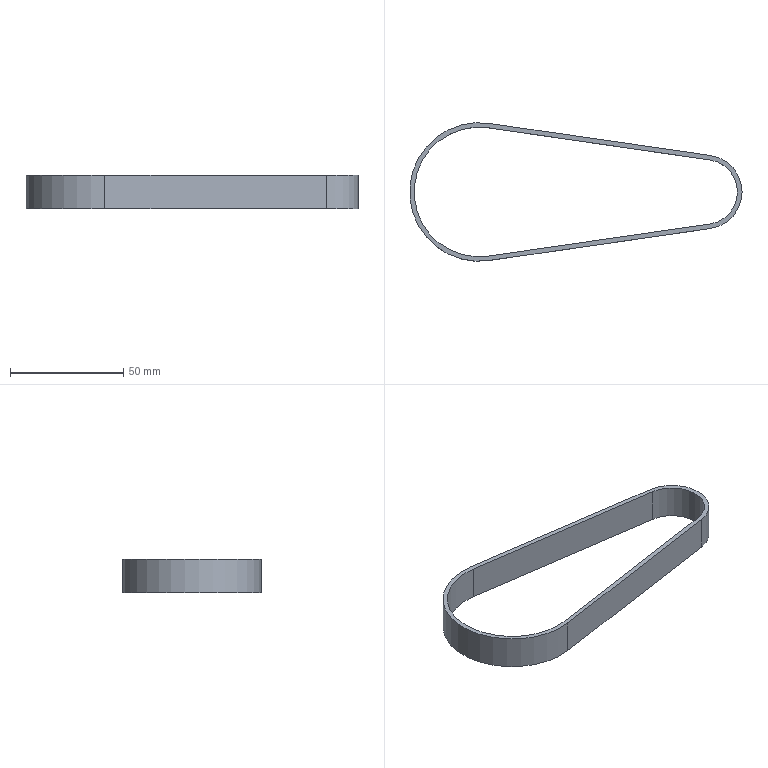Part | NX | 1 solid | 10 faces | box 146.965 x 61.3 x 15 mm | volume 10300 mm3 | plane 6 | cylinder 4 | commonest cylinder face diameters 28.63 x1 32.63 x1 57.3 x1 61.3 x1
STEP:
#1=CARTESIAN_POINT('',(102.339,-16.146,15.));
#2=VERTEX_POINT('',#1);
#3=CARTESIAN_POINT('',(102.339,16.146,15.));
#4=VERTEX_POINT('',#3);
#5=CARTESIAN_POINT('',(100.,0.,15.));
#6=DIRECTION('',(0.,0.,1.));
#7=DIRECTION('',(1.,0.,0.));
#8=AXIS2_PLACEMENT_3D('',#5,#6,#7);
#9=CIRCLE('',#8,16.315);
#10=EDGE_CURVE('',#2,#4,#9,.T.);
#11=ORIENTED_EDGE('',*,*,#10,.T.);
#12=CARTESIAN_POINT('',(4.394,30.333,15.));
#13=VERTEX_POINT('',#12);
#14=CARTESIAN_POINT('',(4.394,30.333,15.));
#15=DIRECTION('',(-0.9897,0.1434,0.));
#16=VECTOR('',#15,1000.);
#17=LINE('',#14,#16);
#18=EDGE_CURVE('',#4,#13,#17,.T.);
#19=ORIENTED_EDGE('',*,*,#18,.T.);
#20=CARTESIAN_POINT('',(4.394,-30.333,15.));
#21=VERTEX_POINT('',#20);
#22=CARTESIAN_POINT('',(0.,0.,15.));
#23=DIRECTION('',(0.,0.,1.));
#24=DIRECTION('',(1.,0.,0.));
#25=AXIS2_PLACEMENT_3D('',#22,#23,#24);
#26=CIRCLE('',#25,30.65);
#27=EDGE_CURVE('',#13,#21,#26,.T.);
#28=ORIENTED_EDGE('',*,*,#27,.T.);
#29=CARTESIAN_POINT('',(4.394,-30.333,15.));
#30=DIRECTION('',(0.9897,0.1434,0.));
#31=VECTOR('',#30,1000.);
#32=LINE('',#29,#31);
#33=EDGE_CURVE('',#21,#2,#32,.T.);
#34=ORIENTED_EDGE('',*,*,#33,.T.);
#35=EDGE_LOOP('',(#11,#19,#28,#34));
#36=FACE_BOUND('',#35,.T.);
#37=CARTESIAN_POINT('',(4.107,-28.354,15.));
#38=VERTEX_POINT('',#37);
#39=CARTESIAN_POINT('',(102.052,-14.167,15.));
#40=VERTEX_POINT('',#39);
#41=CARTESIAN_POINT('',(4.107,-28.354,15.));
#42=DIRECTION('',(0.9897,0.1434,0.));
#43=VECTOR('',#42,1000.);
#44=LINE('',#41,#43);
#45=EDGE_CURVE('',#38,#40,#44,.T.);
#46=ORIENTED_EDGE('',*,*,#45,.F.);
#47=CARTESIAN_POINT('',(4.107,28.354,15.));
#48=VERTEX_POINT('',#47);
#49=CARTESIAN_POINT('',(0.,0.,15.));
#50=DIRECTION('',(0.,0.,1.));
#51=DIRECTION('',(1.,0.,0.));
#52=AXIS2_PLACEMENT_3D('',#49,#50,#51);
#53=CIRCLE('',#52,28.65);
#54=EDGE_CURVE('',#48,#38,#53,.T.);
#55=ORIENTED_EDGE('',*,*,#54,.F.);
#56=CARTESIAN_POINT('',(102.052,14.167,15.));
#57=VERTEX_POINT('',#56);
#58=CARTESIAN_POINT('',(4.107,28.354,15.));
#59=DIRECTION('',(-0.9897,0.1434,0.));
#60=VECTOR('',#59,1000.);
#61=LINE('',#58,#60);
#62=EDGE_CURVE('',#57,#48,#61,.T.);
#63=ORIENTED_EDGE('',*,*,#62,.F.);
#64=CARTESIAN_POINT('',(100.,0.,15.));
#65=DIRECTION('',(0.,0.,1.));
#66=DIRECTION('',(1.,0.,0.));
#67=AXIS2_PLACEMENT_3D('',#64,#65,#66);
#68=CIRCLE('',#67,14.315);
#69=EDGE_CURVE('',#40,#57,#68,.T.);
#70=ORIENTED_EDGE('',*,*,#69,.F.);
#71=EDGE_LOOP('',(#46,#55,#63,#70));
#72=FACE_BOUND('',#71,.T.);
#73=CARTESIAN_POINT('',(100.,0.,15.));
#74=DIRECTION('',(0.,0.,1.));
#75=DIRECTION('',(1.,0.,0.));
#76=AXIS2_PLACEMENT_3D('',#73,#74,#75);
#77=PLANE('',#76);
#78=ADVANCED_FACE('',(#36,#72),#77,.T.);
#79=CARTESIAN_POINT('',(102.339,-16.146,0.));
#80=VERTEX_POINT('',#79);
#81=CARTESIAN_POINT('',(102.339,16.146,0.));
#82=VERTEX_POINT('',#81);
#83=CARTESIAN_POINT('',(100.,0.,0.));
#84=DIRECTION('',(0.,0.,1.));
#85=DIRECTION('',(1.,0.,0.));
#86=AXIS2_PLACEMENT_3D('',#83,#84,#85);
#87=CIRCLE('',#86,16.315);
#88=EDGE_CURVE('',#80,#82,#87,.T.);
#89=ORIENTED_EDGE('',*,*,#88,.F.);
#90=CARTESIAN_POINT('',(4.394,-30.333,0.));
#91=VERTEX_POINT('',#90);
#92=CARTESIAN_POINT('',(4.394,-30.333,0.));
#93=DIRECTION('',(0.9897,0.1434,0.));
#94=VECTOR('',#93,1000.);
#95=LINE('',#92,#94);
#96=EDGE_CURVE('',#91,#80,#95,.T.);
#97=ORIENTED_EDGE('',*,*,#96,.F.);
#98=CARTESIAN_POINT('',(4.394,30.333,0.));
#99=VERTEX_POINT('',#98);
#100=CARTESIAN_POINT('',(0.,0.,0.));
#101=DIRECTION('',(0.,0.,1.));
#102=DIRECTION('',(1.,0.,0.));
#103=AXIS2_PLACEMENT_3D('',#100,#101,#102);
#104=CIRCLE('',#103,30.65);
#105=EDGE_CURVE('',#99,#91,#104,.T.);
#106=ORIENTED_EDGE('',*,*,#105,.F.);
#107=CARTESIAN_POINT('',(4.394,30.333,0.));
#108=DIRECTION('',(-0.9897,0.1434,0.));
#109=VECTOR('',#108,1000.);
#110=LINE('',#107,#109);
#111=EDGE_CURVE('',#82,#99,#110,.T.);
#112=ORIENTED_EDGE('',*,*,#111,.F.);
#113=EDGE_LOOP('',(#89,#97,#106,#112));
#114=FACE_BOUND('',#113,.T.);
#115=CARTESIAN_POINT('',(4.107,28.354,0.));
#116=VERTEX_POINT('',#115);
#117=CARTESIAN_POINT('',(4.107,-28.354,0.));
#118=VERTEX_POINT('',#117);
#119=CARTESIAN_POINT('',(0.,0.,0.));
#120=DIRECTION('',(0.,0.,1.));
#121=DIRECTION('',(1.,0.,0.));
#122=AXIS2_PLACEMENT_3D('',#119,#120,#121);
#123=CIRCLE('',#122,28.65);
#124=EDGE_CURVE('',#116,#118,#123,.T.);
#125=ORIENTED_EDGE('',*,*,#124,.T.);
#126=CARTESIAN_POINT('',(102.052,-14.167,0.));
#127=VERTEX_POINT('',#126);
#128=CARTESIAN_POINT('',(4.107,-28.354,0.));
#129=DIRECTION('',(0.9897,0.1434,0.));
#130=VECTOR('',#129,1000.);
#131=LINE('',#128,#130);
#132=EDGE_CURVE('',#118,#127,#131,.T.);
#133=ORIENTED_EDGE('',*,*,#132,.T.);
#134=CARTESIAN_POINT('',(102.052,14.167,0.));
#135=VERTEX_POINT('',#134);
#136=CARTESIAN_POINT('',(100.,0.,0.));
#137=DIRECTION('',(0.,0.,1.));
#138=DIRECTION('',(1.,0.,0.));
#139=AXIS2_PLACEMENT_3D('',#136,#137,#138);
#140=CIRCLE('',#139,14.315);
#141=EDGE_CURVE('',#127,#135,#140,.T.);
#142=ORIENTED_EDGE('',*,*,#141,.T.);
#143=CARTESIAN_POINT('',(4.107,28.354,0.));
#144=DIRECTION('',(-0.9897,0.1434,0.));
#145=VECTOR('',#144,1000.);
#146=LINE('',#143,#145);
#147=EDGE_CURVE('',#135,#116,#146,.T.);
#148=ORIENTED_EDGE('',*,*,#147,.T.);
#149=EDGE_LOOP('',(#125,#133,#142,#148));
#150=FACE_BOUND('',#149,.T.);
#151=CARTESIAN_POINT('',(100.,0.,0.));
#152=DIRECTION('',(0.,0.,1.));
#153=DIRECTION('',(1.,0.,0.));
#154=AXIS2_PLACEMENT_3D('',#151,#152,#153);
#155=PLANE('',#154);
#156=ADVANCED_FACE('',(#114,#150),#155,.F.);
#157=ORIENTED_EDGE('',*,*,#88,.T.);
#158=CARTESIAN_POINT('',(102.339,16.146,15.));
#159=DIRECTION('',(0.,0.,-1.));
#160=VECTOR('',#159,1000.);
#161=LINE('',#158,#160);
#162=EDGE_CURVE('',#4,#82,#161,.T.);
#163=ORIENTED_EDGE('',*,*,#162,.F.);
#164=ORIENTED_EDGE('',*,*,#10,.F.);
#165=CARTESIAN_POINT('',(102.339,-16.146,15.));
#166=DIRECTION('',(0.,0.,-1.));
#167=VECTOR('',#166,1000.);
#168=LINE('',#165,#167);
#169=EDGE_CURVE('',#2,#80,#168,.T.);
#170=ORIENTED_EDGE('',*,*,#169,.T.);
#171=EDGE_LOOP('',(#157,#163,#164,#170));
#172=FACE_BOUND('',#171,.T.);
#173=CARTESIAN_POINT('',(100.,0.,15.));
#174=DIRECTION('',(0.,0.,-1.));
#175=DIRECTION('',(-1.,0.,0.));
#176=AXIS2_PLACEMENT_3D('',#173,#174,#175);
#177=CYLINDRICAL_SURFACE('',#176,16.315);
#178=ADVANCED_FACE('',(#172),#177,.T.);
#179=ORIENTED_EDGE('',*,*,#111,.T.);
#180=CARTESIAN_POINT('',(4.394,30.333,15.));
#181=DIRECTION('',(0.,0.,-1.));
#182=VECTOR('',#181,1000.);
#183=LINE('',#180,#182);
#184=EDGE_CURVE('',#13,#99,#183,.T.);
#185=ORIENTED_EDGE('',*,*,#184,.F.);
#186=ORIENTED_EDGE('',*,*,#18,.F.);
#187=ORIENTED_EDGE('',*,*,#162,.T.);
#188=EDGE_LOOP('',(#179,#185,#186,#187));
#189=FACE_BOUND('',#188,.T.);
#190=CARTESIAN_POINT('',(4.394,30.333,15.));
#191=DIRECTION('',(-0.1434,-0.9897,0.));
#192=DIRECTION('',(0.9897,-0.1434,0.));
#193=AXIS2_PLACEMENT_3D('',#190,#191,#192);
#194=PLANE('',#193);
#195=ADVANCED_FACE('',(#189),#194,.F.);
#196=ORIENTED_EDGE('',*,*,#105,.T.);
#197=CARTESIAN_POINT('',(4.394,-30.333,15.));
#198=DIRECTION('',(0.,0.,-1.));
#199=VECTOR('',#198,1000.);
#200=LINE('',#197,#199);
#201=EDGE_CURVE('',#21,#91,#200,.T.);
#202=ORIENTED_EDGE('',*,*,#201,.F.);
#203=ORIENTED_EDGE('',*,*,#27,.F.);
#204=ORIENTED_EDGE('',*,*,#184,.T.);
#205=EDGE_LOOP('',(#196,#202,#203,#204));
#206=FACE_BOUND('',#205,.T.);
#207=CARTESIAN_POINT('',(0.,0.,15.));
#208=DIRECTION('',(0.,0.,-1.));
#209=DIRECTION('',(-1.,0.,0.));
#210=AXIS2_PLACEMENT_3D('',#207,#208,#209);
#211=CYLINDRICAL_SURFACE('',#210,30.65);
#212=ADVANCED_FACE('',(#206),#211,.T.);
#213=ORIENTED_EDGE('',*,*,#96,.T.);
#214=ORIENTED_EDGE('',*,*,#169,.F.);
#215=ORIENTED_EDGE('',*,*,#33,.F.);
#216=ORIENTED_EDGE('',*,*,#201,.T.);
#217=EDGE_LOOP('',(#213,#214,#215,#216));
#218=FACE_BOUND('',#217,.T.);
#219=CARTESIAN_POINT('',(4.394,-30.333,15.));
#220=DIRECTION('',(-0.1434,0.9897,0.));
#221=DIRECTION('',(-0.9897,-0.1434,0.));
#222=AXIS2_PLACEMENT_3D('',#219,#220,#221);
#223=PLANE('',#222);
#224=ADVANCED_FACE('',(#218),#223,.F.);
#225=ORIENTED_EDGE('',*,*,#124,.F.);
#226=CARTESIAN_POINT('',(4.107,28.354,15.));
#227=DIRECTION('',(0.,0.,-1.));
#228=VECTOR('',#227,1000.);
#229=LINE('',#226,#228);
#230=EDGE_CURVE('',#48,#116,#229,.T.);
#231=ORIENTED_EDGE('',*,*,#230,.F.);
#232=ORIENTED_EDGE('',*,*,#54,.T.);
#233=CARTESIAN_POINT('',(4.107,-28.354,15.));
#234=DIRECTION('',(0.,0.,-1.));
#235=VECTOR('',#234,1000.);
#236=LINE('',#233,#235);
#237=EDGE_CURVE('',#38,#118,#236,.T.);
#238=ORIENTED_EDGE('',*,*,#237,.T.);
#239=EDGE_LOOP('',(#225,#231,#232,#238));
#240=FACE_BOUND('',#239,.T.);
#241=CARTESIAN_POINT('',(0.,0.,15.));
#242=DIRECTION('',(0.,0.,-1.));
#243=DIRECTION('',(-1.,0.,0.));
#244=AXIS2_PLACEMENT_3D('',#241,#242,#243);
#245=CYLINDRICAL_SURFACE('',#244,28.65);
#246=ADVANCED_FACE('',(#240),#245,.F.);
#247=ORIENTED_EDGE('',*,*,#132,.F.);
#248=ORIENTED_EDGE('',*,*,#237,.F.);
#249=ORIENTED_EDGE('',*,*,#45,.T.);
#250=CARTESIAN_POINT('',(102.052,-14.167,15.));
#251=DIRECTION('',(0.,0.,-1.));
#252=VECTOR('',#251,1000.);
#253=LINE('',#250,#252);
#254=EDGE_CURVE('',#40,#127,#253,.T.);
#255=ORIENTED_EDGE('',*,*,#254,.T.);
#256=EDGE_LOOP('',(#247,#248,#249,#255));
#257=FACE_BOUND('',#256,.T.);
#258=CARTESIAN_POINT('',(4.107,-28.354,15.));
#259=DIRECTION('',(-0.1434,0.9897,0.));
#260=DIRECTION('',(-0.9897,-0.1434,0.));
#261=AXIS2_PLACEMENT_3D('',#258,#259,#260);
#262=PLANE('',#261);
#263=ADVANCED_FACE('',(#257),#262,.T.);
#264=ORIENTED_EDGE('',*,*,#141,.F.);
#265=ORIENTED_EDGE('',*,*,#254,.F.);
#266=ORIENTED_EDGE('',*,*,#69,.T.);
#267=CARTESIAN_POINT('',(102.052,14.167,15.));
#268=DIRECTION('',(0.,0.,-1.));
#269=VECTOR('',#268,1000.);
#270=LINE('',#267,#269);
#271=EDGE_CURVE('',#57,#135,#270,.T.);
#272=ORIENTED_EDGE('',*,*,#271,.T.);
#273=EDGE_LOOP('',(#264,#265,#266,#272));
#274=FACE_BOUND('',#273,.T.);
#275=CARTESIAN_POINT('',(100.,0.,15.));
#276=DIRECTION('',(0.,0.,-1.));
#277=DIRECTION('',(-1.,0.,0.));
#278=AXIS2_PLACEMENT_3D('',#275,#276,#277);
#279=CYLINDRICAL_SURFACE('',#278,14.315);
#280=ADVANCED_FACE('',(#274),#279,.F.);
#281=ORIENTED_EDGE('',*,*,#147,.F.);
#282=ORIENTED_EDGE('',*,*,#271,.F.);
#283=ORIENTED_EDGE('',*,*,#62,.T.);
#284=ORIENTED_EDGE('',*,*,#230,.T.);
#285=EDGE_LOOP('',(#281,#282,#283,#284));
#286=FACE_BOUND('',#285,.T.);
#287=CARTESIAN_POINT('',(4.107,28.354,15.));
#288=DIRECTION('',(-0.1434,-0.9897,0.));
#289=DIRECTION('',(0.9897,-0.1434,0.));
#290=AXIS2_PLACEMENT_3D('',#287,#288,#289);
#291=PLANE('',#290);
#292=ADVANCED_FACE('',(#286),#291,.T.);
#293=CLOSED_SHELL('',(#78,#156,#178,#195,#212,#224,#246,#263,#280,#292));
#294=MANIFOLD_SOLID_BREP('',#293);
#295=(LENGTH_UNIT()NAMED_UNIT(*)SI_UNIT(.MILLI.,.METRE.));
#296=UNCERTAINTY_MEASURE_WITH_UNIT(LENGTH_MEASURE(0.00001),#295,'','');
#297=(NAMED_UNIT(*)PLANE_ANGLE_UNIT()SI_UNIT($,.RADIAN.));
#298=(NAMED_UNIT(*)SI_UNIT($,.STERADIAN.)SOLID_ANGLE_UNIT());
#299=(GEOMETRIC_REPRESENTATION_CONTEXT(3)GLOBAL_UNCERTAINTY_ASSIGNED_CONTEXT((#296))GLOBAL_UNIT_ASSIGNED_CONTEXT((#295,#297,#298))REPRESENTATION_CONTEXT('',''));
#300=ADVANCED_BREP_SHAPE_REPRESENTATION('',(#294),#299);